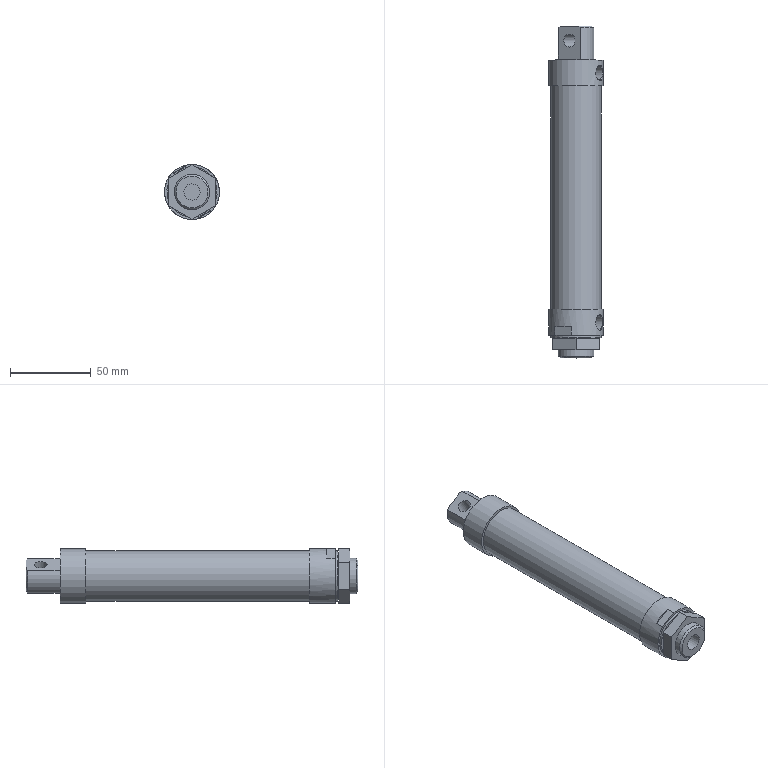Part | NX | features WGN01-25-100-Y-2-001 2 | 1 solid | 41 faces | box 34 x 205 x 34 mm | volume 131750 mm3 | plane 22 | cylinder 12 | cone 7 | commonest cylinder face diameters 22 x4 8.566 x2 31 x2 34 x2 8 x1 10 x1
STEP:
#1=CARTESIAN_POINT('',(-5.5,333.716,144.407));
#2=VERTEX_POINT('',#1);
#3=CARTESIAN_POINT('',(-0.000000942,333.716,134.881));
#4=DIRECTION('',(0.,1.,0.));
#5=DIRECTION('',(-0.5,0.,0.866));
#6=AXIS2_PLACEMENT_3D('',#3,#4,#5);
#7=CIRCLE('',#6,11.);
#8=EDGE_CURVE('',#2,#2,#7,.T.);
#9=ORIENTED_EDGE('',*,*,#8,.F.);
#10=EDGE_LOOP('',(#9));
#11=FACE_BOUND('',#10,.T.);
#12=CARTESIAN_POINT('',(-5.5,329.847,144.407));
#13=VERTEX_POINT('',#12);
#14=CARTESIAN_POINT('',(-0.000000942,329.847,134.881));
#15=DIRECTION('',(0.,1.,0.));
#16=DIRECTION('',(-0.5,0.,0.866));
#17=AXIS2_PLACEMENT_3D('',#14,#15,#16);
#18=CIRCLE('',#17,11.);
#19=EDGE_CURVE('',#13,#13,#18,.T.);
#20=ORIENTED_EDGE('',*,*,#19,.T.);
#21=EDGE_LOOP('',(#20));
#22=FACE_BOUND('',#21,.T.);
#23=CARTESIAN_POINT('',(-0.000000942,342.716,134.881));
#24=DIRECTION('',(0.,1.,0.));
#25=DIRECTION('',(0.5,0.,-0.866));
#26=AXIS2_PLACEMENT_3D('',#23,#24,#25);
#27=CYLINDRICAL_SURFACE('',#26,11.);
#28=ADVANCED_FACE('',(#11,#22),#27,.T.);
#29=ORIENTED_EDGE('',*,*,#19,.F.);
#30=EDGE_LOOP('',(#29));
#31=FACE_BOUND('',#30,.T.);
#32=CARTESIAN_POINT('',(-4.934,328.716,143.428));
#33=VERTEX_POINT('',#32);
#34=CARTESIAN_POINT('',(-0.000000942,328.716,134.881));
#35=DIRECTION('',(0.,1.,0.));
#36=DIRECTION('',(-0.5,0.,0.866));
#37=AXIS2_PLACEMENT_3D('',#34,#35,#36);
#38=CIRCLE('',#37,9.869);
#39=EDGE_CURVE('',#33,#33,#38,.T.);
#40=ORIENTED_EDGE('',*,*,#39,.T.);
#41=EDGE_LOOP('',(#40));
#42=FACE_BOUND('',#41,.T.);
#43=CARTESIAN_POINT('',(-0.000000942,328.716,134.881));
#44=DIRECTION('',(0.,1.,0.));
#45=DIRECTION('',(0.5,0.,-0.866));
#46=AXIS2_PLACEMENT_3D('',#43,#44,#45);
#47=CONICAL_SURFACE('',#46,9.869,0.7854);
#48=ADVANCED_FACE('',(#31,#42),#47,.T.);
#49=CARTESIAN_POINT('',(-2.5,512.716,139.211));
#50=VERTEX_POINT('',#49);
#51=CARTESIAN_POINT('',(-0.000000942,512.716,134.881));
#52=DIRECTION('',(0.,1.,0.));
#53=DIRECTION('',(-0.5,0.,0.866));
#54=AXIS2_PLACEMENT_3D('',#51,#52,#53);
#55=CIRCLE('',#54,5.);
#56=EDGE_CURVE('',#50,#50,#55,.T.);
#57=ORIENTED_EDGE('',*,*,#56,.T.);
#58=EDGE_LOOP('',(#57));
#59=FACE_BOUND('',#58,.T.);
#60=CARTESIAN_POINT('',(-2.5,328.716,139.211));
#61=VERTEX_POINT('',#60);
#62=CARTESIAN_POINT('',(-0.000000942,328.716,134.881));
#63=DIRECTION('',(0.,1.,0.));
#64=DIRECTION('',(-0.5,0.,0.866));
#65=AXIS2_PLACEMENT_3D('',#62,#63,#64);
#66=CIRCLE('',#65,5.);
#67=EDGE_CURVE('',#61,#61,#66,.T.);
#68=ORIENTED_EDGE('',*,*,#67,.F.);
#69=EDGE_LOOP('',(#68));
#70=FACE_BOUND('',#69,.T.);
#71=CARTESIAN_POINT('',(-0.000000942,512.716,134.881));
#72=DIRECTION('',(0.,1.,0.));
#73=DIRECTION('',(0.5,0.,-0.866));
#74=AXIS2_PLACEMENT_3D('',#71,#72,#73);
#75=CYLINDRICAL_SURFACE('',#74,5.);
#76=ADVANCED_FACE('',(#59,#70),#75,.F.);
#77=CARTESIAN_POINT('',(-7.75,342.716,148.305));
#78=VERTEX_POINT('',#77);
#79=CARTESIAN_POINT('',(-0.000000942,342.716,134.881));
#80=DIRECTION('',(0.,1.,0.));
#81=DIRECTION('',(-0.5,0.,0.866));
#82=AXIS2_PLACEMENT_3D('',#79,#80,#81);
#83=CIRCLE('',#82,15.5);
#84=EDGE_CURVE('',#78,#78,#83,.T.);
#85=ORIENTED_EDGE('',*,*,#84,.F.);
#86=EDGE_LOOP('',(#85));
#87=FACE_BOUND('',#86,.T.);
#88=CARTESIAN_POINT('',(-7.75,341.216,148.305));
#89=VERTEX_POINT('',#88);
#90=CARTESIAN_POINT('',(-0.000000942,341.216,134.881));
#91=DIRECTION('',(0.,1.,0.));
#92=DIRECTION('',(-0.5,0.,0.866));
#93=AXIS2_PLACEMENT_3D('',#90,#91,#92);
#94=CIRCLE('',#93,15.5);
#95=EDGE_CURVE('',#89,#89,#94,.T.);
#96=ORIENTED_EDGE('',*,*,#95,.T.);
#97=EDGE_LOOP('',(#96));
#98=FACE_BOUND('',#97,.T.);
#99=CARTESIAN_POINT('',(-0.000000942,342.716,134.881));
#100=DIRECTION('',(0.,1.,0.));
#101=DIRECTION('',(0.5,0.,-0.866));
#102=AXIS2_PLACEMENT_3D('',#99,#100,#101);
#103=CYLINDRICAL_SURFACE('',#102,15.5);
#104=ADVANCED_FACE('',(#87,#98),#103,.T.);
#105=CARTESIAN_POINT('',(-5.5,341.216,144.407));
#106=VERTEX_POINT('',#105);
#107=CARTESIAN_POINT('',(-0.000000942,341.216,134.881));
#108=DIRECTION('',(0.,1.,0.));
#109=DIRECTION('',(-0.5,0.,0.866));
#110=AXIS2_PLACEMENT_3D('',#107,#108,#109);
#111=CIRCLE('',#110,11.);
#112=EDGE_CURVE('',#106,#106,#111,.T.);
#113=ORIENTED_EDGE('',*,*,#112,.F.);
#114=EDGE_LOOP('',(#113));
#115=FACE_BOUND('',#114,.T.);
#116=CARTESIAN_POINT('',(-5.5,340.716,144.407));
#117=VERTEX_POINT('',#116);
#118=CARTESIAN_POINT('',(-0.000000942,340.716,134.881));
#119=DIRECTION('',(0.,1.,0.));
#120=DIRECTION('',(-0.5,0.,0.866));
#121=AXIS2_PLACEMENT_3D('',#118,#119,#120);
#122=CIRCLE('',#121,11.);
#123=EDGE_CURVE('',#117,#117,#122,.T.);
#124=ORIENTED_EDGE('',*,*,#123,.T.);
#125=EDGE_LOOP('',(#124));
#126=FACE_BOUND('',#125,.T.);
#127=CARTESIAN_POINT('',(-0.000000942,342.716,134.881));
#128=DIRECTION('',(0.,1.,0.));
#129=DIRECTION('',(0.5,0.,-0.866));
#130=AXIS2_PLACEMENT_3D('',#127,#128,#129);
#131=CYLINDRICAL_SURFACE('',#130,11.);
#132=ADVANCED_FACE('',(#115,#126),#131,.T.);
#133=CARTESIAN_POINT('',(-4.,520.716,141.809));
#134=VERTEX_POINT('',#133);
#135=CARTESIAN_POINT('',(-4.,524.716,141.809));
#136=DIRECTION('',(-0.5,0.,0.866));
#137=DIRECTION('',(0.,-1.,0.));
#138=AXIS2_PLACEMENT_3D('',#135,#136,#137);
#139=CIRCLE('',#138,4.);
#140=EDGE_CURVE('',#134,#134,#139,.T.);
#141=ORIENTED_EDGE('',*,*,#140,.T.);
#142=EDGE_LOOP('',(#141));
#143=FACE_BOUND('',#142,.T.);
#144=CARTESIAN_POINT('',(4.,520.716,127.953));
#145=VERTEX_POINT('',#144);
#146=CARTESIAN_POINT('',(4.,524.716,127.953));
#147=DIRECTION('',(-0.5,0.,0.866));
#148=DIRECTION('',(0.,-1.,0.));
#149=AXIS2_PLACEMENT_3D('',#146,#147,#148);
#150=CIRCLE('',#149,4.);
#151=EDGE_CURVE('',#145,#145,#150,.F.);
#152=ORIENTED_EDGE('',*,*,#151,.T.);
#153=EDGE_LOOP('',(#152));
#154=FACE_BOUND('',#153,.T.);
#155=CARTESIAN_POINT('',(11.,524.716,115.829));
#156=DIRECTION('',(-0.5,0.,0.866));
#157=DIRECTION('',(0.,1.,0.));
#158=AXIS2_PLACEMENT_3D('',#155,#156,#157);
#159=CYLINDRICAL_SURFACE('',#158,4.);
#160=ADVANCED_FACE('',(#143,#154),#159,.F.);
#161=CARTESIAN_POINT('',(16.396,504.716,139.372));
#162=VERTEX_POINT('',#161);
#163=CARTESIAN_POINT('',(16.248,507.739,139.997));
#164=CARTESIAN_POINT('',(16.495,504.71,138.957));
#165=CARTESIAN_POINT('',(16.248,501.709,139.993));
#166=CARTESIAN_POINT('',(15.571,500.158,141.771));
#167=CARTESIAN_POINT('',(14.763,499.703,143.38));
#168=CARTESIAN_POINT('',(13.772,500.14,144.894));
#169=CARTESIAN_POINT('',(12.557,501.689,146.391));
#170=CARTESIAN_POINT('',(11.777,504.707,147.128));
#171=CARTESIAN_POINT('',(12.548,507.718,146.4));
#172=CARTESIAN_POINT('',(13.751,509.272,144.923));
#173=CARTESIAN_POINT('',(14.741,509.729,143.417));
#174=CARTESIAN_POINT('',(15.559,509.291,141.8));
#175=CARTESIAN_POINT('',(16.248,507.739,139.997));
#176=CARTESIAN_POINT('',(16.495,504.71,138.957));
#177=CARTESIAN_POINT('',(16.248,501.709,139.993));
#178=B_SPLINE_CURVE_WITH_KNOTS('',3,(#163,#164,#165,#166,#167,#168,#169,#170,#171,#172,#173,#174,#175,#176,#177),.UNSPECIFIED.,.T.,.F.,(1,1,1,1,1,1,1,1,1,1,1,1,1,1,1,1,1,1,1),(-0.007178,-0.005384,-0.003589,0.,0.003589,0.005384,0.007178,0.008973,0.01077,0.01436,0.01795,0.01974,0.02154,0.02333,0.02512,0.02871,0.0323,0.0341,0.03589),.UNSPECIFIED.);
#179=EDGE_CURVE('',#162,#162,#178,.T.);
#180=ORIENTED_EDGE('',*,*,#179,.F.);
#181=EDGE_LOOP('',(#180));
#182=FACE_BOUND('',#181,.T.);
#183=CARTESIAN_POINT('',(16.361,504.716,139.382));
#184=VERTEX_POINT('',#183);
#185=CARTESIAN_POINT('',(14.219,504.716,143.091));
#186=DIRECTION('',(0.866,0.,0.5));
#187=DIRECTION('',(0.5,0.,-0.866));
#188=AXIS2_PLACEMENT_3D('',#185,#186,#187);
#189=CIRCLE('',#188,4.283);
#190=EDGE_CURVE('',#184,#184,#189,.T.);
#191=ORIENTED_EDGE('',*,*,#190,.F.);
#192=EDGE_LOOP('',(#191));
#193=FACE_BOUND('',#192,.T.);
#194=CARTESIAN_POINT('',(14.219,504.716,143.091));
#195=DIRECTION('',(0.866,0.,0.5));
#196=DIRECTION('',(-0.5,0.,0.866));
#197=AXIS2_PLACEMENT_3D('',#194,#195,#196);
#198=CONICAL_SURFACE('',#197,4.283,0.7854);
#199=ADVANCED_FACE('',(#182,#193),#198,.F.);
#200=ORIENTED_EDGE('',*,*,#190,.T.);
#201=EDGE_LOOP('',(#200));
#202=FACE_BOUND('',#201,.T.);
#203=CARTESIAN_POINT('',(9.503,504.716,135.422));
#204=VERTEX_POINT('',#203);
#205=CARTESIAN_POINT('',(7.361,504.716,139.131));
#206=DIRECTION('',(0.866,0.,0.5));
#207=DIRECTION('',(0.5,0.,-0.866));
#208=AXIS2_PLACEMENT_3D('',#205,#206,#207);
#209=CIRCLE('',#208,4.283);
#210=EDGE_CURVE('',#204,#204,#209,.T.);
#211=ORIENTED_EDGE('',*,*,#210,.F.);
#212=EDGE_LOOP('',(#211));
#213=FACE_BOUND('',#212,.T.);
#214=CARTESIAN_POINT('',(14.722,504.716,143.381));
#215=DIRECTION('',(0.866,0.,0.5));
#216=DIRECTION('',(-0.5,0.,0.866));
#217=AXIS2_PLACEMENT_3D('',#214,#215,#216);
#218=CYLINDRICAL_SURFACE('',#217,4.283);
#219=ADVANCED_FACE('',(#202,#213),#218,.F.);
#220=ORIENTED_EDGE('',*,*,#210,.T.);
#221=EDGE_LOOP('',(#220));
#222=FACE_BOUND('',#221,.T.);
#223=CARTESIAN_POINT('',(5.22,504.716,137.895));
#224=VERTEX_POINT('',#223);
#225=VERTEX_LOOP('',#224);
#226=FACE_BOUND('',#225,.T.);
#227=CARTESIAN_POINT('',(871.245,504.716,637.895));
#228=DIRECTION('',(0.866,0.,0.5));
#229=DIRECTION('',(-0.5,0.,0.866));
#230=AXIS2_PLACEMENT_3D('',#227,#228,#229);
#231=CONICAL_SURFACE('',#230,1732.051,1.047);
#232=ADVANCED_FACE('',(#222,#226),#231,.F.);
#233=CARTESIAN_POINT('',(5.22,350.716,142.84));
#234=VERTEX_POINT('',#233);
#235=CARTESIAN_POINT('',(7.361,350.716,139.131));
#236=DIRECTION('',(-0.866,0.,-0.5));
#237=DIRECTION('',(-0.5,0.,0.866));
#238=AXIS2_PLACEMENT_3D('',#235,#236,#237);
#239=CIRCLE('',#238,4.283);
#240=EDGE_CURVE('',#234,#234,#239,.T.);
#241=ORIENTED_EDGE('',*,*,#240,.F.);
#242=EDGE_LOOP('',(#241));
#243=FACE_BOUND('',#242,.T.);
#244=CARTESIAN_POINT('',(5.22,350.716,137.895));
#245=VERTEX_POINT('',#244);
#246=VERTEX_LOOP('',#245);
#247=FACE_BOUND('',#246,.T.);
#248=CARTESIAN_POINT('',(7.361,350.716,139.131));
#249=DIRECTION('',(0.866,0.,0.5));
#250=DIRECTION('',(-0.5,0.,0.866));
#251=AXIS2_PLACEMENT_3D('',#248,#249,#250);
#252=CONICAL_SURFACE('',#251,4.283,1.047);
#253=ADVANCED_FACE('',(#243,#247),#252,.F.);
#254=ORIENTED_EDGE('',*,*,#240,.T.);
#255=EDGE_LOOP('',(#254));
#256=FACE_BOUND('',#255,.T.);
#257=CARTESIAN_POINT('',(16.361,350.716,139.382));
#258=VERTEX_POINT('',#257);
#259=CARTESIAN_POINT('',(14.219,350.716,143.091));
#260=DIRECTION('',(0.866,0.,0.5));
#261=DIRECTION('',(0.5,0.,-0.866));
#262=AXIS2_PLACEMENT_3D('',#259,#260,#261);
#263=CIRCLE('',#262,4.283);
#264=EDGE_CURVE('',#258,#258,#263,.F.);
#265=ORIENTED_EDGE('',*,*,#264,.F.);
#266=EDGE_LOOP('',(#265));
#267=FACE_BOUND('',#266,.T.);
#268=CARTESIAN_POINT('',(7.361,350.716,139.131));
#269=DIRECTION('',(-0.866,0.,-0.5));
#270=DIRECTION('',(0.5,0.,-0.866));
#271=AXIS2_PLACEMENT_3D('',#268,#269,#270);
#272=CYLINDRICAL_SURFACE('',#271,4.283);
#273=ADVANCED_FACE('',(#256,#267),#272,.F.);
#274=CARTESIAN_POINT('',(16.396,350.716,139.372));
#275=VERTEX_POINT('',#274);
#276=CARTESIAN_POINT('',(16.248,353.739,139.997));
#277=CARTESIAN_POINT('',(16.495,350.71,138.957));
#278=CARTESIAN_POINT('',(16.248,347.709,139.993));
#279=CARTESIAN_POINT('',(15.571,346.158,141.771));
#280=CARTESIAN_POINT('',(14.763,345.703,143.38));
#281=CARTESIAN_POINT('',(13.772,346.14,144.894));
#282=CARTESIAN_POINT('',(12.557,347.689,146.391));
#283=CARTESIAN_POINT('',(11.777,350.707,147.128));
#284=CARTESIAN_POINT('',(12.548,353.718,146.4));
#285=CARTESIAN_POINT('',(13.751,355.272,144.923));
#286=CARTESIAN_POINT('',(14.741,355.729,143.417));
#287=CARTESIAN_POINT('',(15.559,355.291,141.8));
#288=CARTESIAN_POINT('',(16.248,353.739,139.997));
#289=CARTESIAN_POINT('',(16.495,350.71,138.957));
#290=CARTESIAN_POINT('',(16.248,347.709,139.993));
#291=B_SPLINE_CURVE_WITH_KNOTS('',3,(#276,#277,#278,#279,#280,#281,#282,#283,#284,#285,#286,#287,#288,#289,#290),.UNSPECIFIED.,.T.,.F.,(1,1,1,1,1,1,1,1,1,1,1,1,1,1,1,1,1,1,1),(-0.007178,-0.005384,-0.003589,0.,0.003589,0.005384,0.007178,0.008973,0.01077,0.01436,0.01795,0.01974,0.02154,0.02333,0.02512,0.02871,0.0323,0.0341,0.03589),.UNSPECIFIED.);
#292=EDGE_CURVE('',#275,#275,#291,.T.);
#293=ORIENTED_EDGE('',*,*,#292,.F.);
#294=EDGE_LOOP('',(#293));
#295=FACE_BOUND('',#294,.T.);
#296=ORIENTED_EDGE('',*,*,#264,.T.);
#297=EDGE_LOOP('',(#296));
#298=FACE_BOUND('',#297,.T.);
#299=CARTESIAN_POINT('',(14.722,350.716,143.381));
#300=DIRECTION('',(0.866,0.,0.5));
#301=DIRECTION('',(-0.5,0.,0.866));
#302=AXIS2_PLACEMENT_3D('',#299,#300,#301);
#303=CONICAL_SURFACE('',#302,4.864,0.7854);
#304=ADVANCED_FACE('',(#295,#298),#303,.F.);
#305=CARTESIAN_POINT('',(-7.75,496.716,148.305));
#306=VERTEX_POINT('',#305);
#307=CARTESIAN_POINT('',(-0.000000942,496.716,134.881));
#308=DIRECTION('',(0.,1.,0.));
#309=DIRECTION('',(-0.5,0.,0.866));
#310=AXIS2_PLACEMENT_3D('',#307,#308,#309);
#311=CIRCLE('',#310,15.5);
#312=EDGE_CURVE('',#306,#306,#311,.T.);
#313=ORIENTED_EDGE('',*,*,#312,.F.);
#314=EDGE_LOOP('',(#313));
#315=FACE_BOUND('',#314,.T.);
#316=CARTESIAN_POINT('',(-7.75,358.716,148.305));
#317=VERTEX_POINT('',#316);
#318=CARTESIAN_POINT('',(-0.000000942,358.716,134.881));
#319=DIRECTION('',(0.,1.,0.));
#320=DIRECTION('',(-0.5,0.,0.866));
#321=AXIS2_PLACEMENT_3D('',#318,#319,#320);
#322=CIRCLE('',#321,15.5);
#323=EDGE_CURVE('',#317,#317,#322,.T.);
#324=ORIENTED_EDGE('',*,*,#323,.T.);
#325=EDGE_LOOP('',(#324));
#326=FACE_BOUND('',#325,.T.);
#327=CARTESIAN_POINT('',(-0.000000942,512.716,134.881));
#328=DIRECTION('',(0.,1.,0.));
#329=DIRECTION('',(0.5,0.,-0.866));
#330=AXIS2_PLACEMENT_3D('',#327,#328,#329);
#331=CYLINDRICAL_SURFACE('',#330,15.5);
#332=ADVANCED_FACE('',(#315,#326),#331,.T.);
#333=CARTESIAN_POINT('',(-8.5,358.716,149.604));
#334=VERTEX_POINT('',#333);
#335=CARTESIAN_POINT('',(-0.000000942,358.716,134.881));
#336=DIRECTION('',(0.,1.,0.));
#337=DIRECTION('',(-0.5,0.,0.866));
#338=AXIS2_PLACEMENT_3D('',#335,#336,#337);
#339=CIRCLE('',#338,17.);
#340=EDGE_CURVE('',#334,#334,#339,.T.);
#341=ORIENTED_EDGE('',*,*,#340,.F.);
#342=EDGE_LOOP('',(#341));
#343=FACE_BOUND('',#342,.T.);
#344=ORIENTED_EDGE('',*,*,#292,.T.);
#345=EDGE_LOOP('',(#344));
#346=FACE_BOUND('',#345,.T.);
#347=CARTESIAN_POINT('',(12.975,348.049,123.897));
#348=VERTEX_POINT('',#347);
#349=CARTESIAN_POINT('',(3.025,348.049,118.153));
#350=VERTEX_POINT('',#349);
#351=CARTESIAN_POINT('',(-0.000000942,348.049,134.881));
#352=DIRECTION('',(0.,1.,0.));
#353=DIRECTION('',(0.7632,0.,-0.6461));
#354=AXIS2_PLACEMENT_3D('',#351,#352,#353);
#355=CIRCLE('',#354,17.);
#356=EDGE_CURVE('',#348,#350,#355,.T.);
#357=ORIENTED_EDGE('',*,*,#356,.T.);
#358=CARTESIAN_POINT('',(3.025,342.716,118.153));
#359=VERTEX_POINT('',#358);
#360=CARTESIAN_POINT('',(3.025,348.049,118.153));
#361=DIRECTION('',(0.,-1.,0.));
#362=VECTOR('',#361,1000.);
#363=LINE('',#360,#362);
#364=EDGE_CURVE('',#359,#350,#363,.F.);
#365=ORIENTED_EDGE('',*,*,#364,.F.);
#366=CARTESIAN_POINT('',(-12.975,342.716,145.865));
#367=VERTEX_POINT('',#366);
#368=CARTESIAN_POINT('',(-0.000000942,342.716,134.881));
#369=DIRECTION('',(0.,1.,0.));
#370=DIRECTION('',(0.1779,0.,-0.984));
#371=AXIS2_PLACEMENT_3D('',#368,#369,#370);
#372=CIRCLE('',#371,17.);
#373=EDGE_CURVE('',#359,#367,#372,.T.);
#374=ORIENTED_EDGE('',*,*,#373,.T.);
#375=CARTESIAN_POINT('',(-12.975,348.049,145.865));
#376=VERTEX_POINT('',#375);
#377=CARTESIAN_POINT('',(-12.975,348.049,145.865));
#378=DIRECTION('',(0.,-1.,0.));
#379=VECTOR('',#378,1000.);
#380=LINE('',#377,#379);
#381=EDGE_CURVE('',#367,#376,#380,.F.);
#382=ORIENTED_EDGE('',*,*,#381,.T.);
#383=CARTESIAN_POINT('',(-3.025,348.049,151.61));
#384=VERTEX_POINT('',#383);
#385=CARTESIAN_POINT('',(-0.000000942,348.049,134.881));
#386=DIRECTION('',(0.,1.,0.));
#387=DIRECTION('',(-0.7632,0.,0.6461));
#388=AXIS2_PLACEMENT_3D('',#385,#386,#387);
#389=CIRCLE('',#388,17.);
#390=EDGE_CURVE('',#376,#384,#389,.T.);
#391=ORIENTED_EDGE('',*,*,#390,.T.);
#392=CARTESIAN_POINT('',(-3.025,342.716,151.61));
#393=VERTEX_POINT('',#392);
#394=CARTESIAN_POINT('',(-3.025,348.049,151.61));
#395=DIRECTION('',(0.,-1.,0.));
#396=VECTOR('',#395,1000.);
#397=LINE('',#394,#396);
#398=EDGE_CURVE('',#384,#393,#397,.T.);
#399=ORIENTED_EDGE('',*,*,#398,.T.);
#400=CARTESIAN_POINT('',(12.975,342.716,123.897));
#401=VERTEX_POINT('',#400);
#402=CARTESIAN_POINT('',(-0.000000942,342.716,134.881));
#403=DIRECTION('',(0.,1.,0.));
#404=DIRECTION('',(-0.1779,0.,0.984));
#405=AXIS2_PLACEMENT_3D('',#402,#403,#404);
#406=CIRCLE('',#405,17.);
#407=EDGE_CURVE('',#393,#401,#406,.T.);
#408=ORIENTED_EDGE('',*,*,#407,.T.);
#409=CARTESIAN_POINT('',(12.975,348.049,123.897));
#410=DIRECTION('',(0.,-1.,0.));
#411=VECTOR('',#410,1000.);
#412=LINE('',#409,#411);
#413=EDGE_CURVE('',#348,#401,#412,.T.);
#414=ORIENTED_EDGE('',*,*,#413,.F.);
#415=EDGE_LOOP('',(#357,#365,#374,#382,#391,#399,#408,#414));
#416=FACE_BOUND('',#415,.T.);
#417=CARTESIAN_POINT('',(-0.000000942,512.716,134.881));
#418=DIRECTION('',(0.,1.,0.));
#419=DIRECTION('',(0.5,0.,-0.866));
#420=AXIS2_PLACEMENT_3D('',#417,#418,#419);
#421=CYLINDRICAL_SURFACE('',#420,17.);
#422=ADVANCED_FACE('',(#343,#346,#416),#421,.T.);
#423=CARTESIAN_POINT('',(-8.5,512.716,149.604));
#424=VERTEX_POINT('',#423);
#425=CARTESIAN_POINT('',(-0.000000942,512.716,134.881));
#426=DIRECTION('',(0.,1.,0.));
#427=DIRECTION('',(-0.5,0.,0.866));
#428=AXIS2_PLACEMENT_3D('',#425,#426,#427);
#429=CIRCLE('',#428,17.);
#430=EDGE_CURVE('',#424,#424,#429,.T.);
#431=ORIENTED_EDGE('',*,*,#430,.F.);
#432=EDGE_LOOP('',(#431));
#433=FACE_BOUND('',#432,.T.);
#434=ORIENTED_EDGE('',*,*,#179,.T.);
#435=EDGE_LOOP('',(#434));
#436=FACE_BOUND('',#435,.T.);
#437=CARTESIAN_POINT('',(-8.5,496.716,149.604));
#438=VERTEX_POINT('',#437);
#439=CARTESIAN_POINT('',(-0.000000942,496.716,134.881));
#440=DIRECTION('',(0.,1.,0.));
#441=DIRECTION('',(-0.5,0.,0.866));
#442=AXIS2_PLACEMENT_3D('',#439,#440,#441);
#443=CIRCLE('',#442,17.);
#444=EDGE_CURVE('',#438,#438,#443,.T.);
#445=ORIENTED_EDGE('',*,*,#444,.T.);
#446=EDGE_LOOP('',(#445));
#447=FACE_BOUND('',#446,.T.);
#448=CARTESIAN_POINT('',(-0.000000942,512.716,134.881));
#449=DIRECTION('',(0.,1.,0.));
#450=DIRECTION('',(0.5,0.,-0.866));
#451=AXIS2_PLACEMENT_3D('',#448,#449,#450);
#452=CYLINDRICAL_SURFACE('',#451,17.);
#453=ADVANCED_FACE('',(#433,#436,#447),#452,.T.);
#454=CARTESIAN_POINT('',(-2.538,532.584,124.178));
#455=VERTEX_POINT('',#454);
#456=CARTESIAN_POINT('',(-10.538,532.584,138.034));
#457=VERTEX_POINT('',#456);
#458=CARTESIAN_POINT('',(-0.000000942,532.584,134.881));
#459=DIRECTION('',(0.,1.,0.));
#460=DIRECTION('',(-0.2308,0.,-0.973));
#461=AXIS2_PLACEMENT_3D('',#458,#459,#460);
#462=CIRCLE('',#461,11.);
#463=EDGE_CURVE('',#455,#457,#462,.T.);
#464=ORIENTED_EDGE('',*,*,#463,.T.);
#465=CARTESIAN_POINT('',(-9.004,533.716,138.92));
#466=VERTEX_POINT('',#465);
#467=CARTESIAN_POINT('',(-10.538,532.584,138.034));
#468=CARTESIAN_POINT('',(-10.41,532.686,138.109));
#469=CARTESIAN_POINT('',(-10.218,532.836,138.219));
#470=CARTESIAN_POINT('',(-9.997,533.004,138.347));
#471=CARTESIAN_POINT('',(-9.888,533.086,138.41));
#472=CARTESIAN_POINT('',(-9.841,533.121,138.437));
#473=CARTESIAN_POINT('',(-9.81,533.144,138.455));
#474=CARTESIAN_POINT('',(-9.795,533.155,138.464));
#475=CARTESIAN_POINT('',(-9.515,533.362,138.625));
#476=CARTESIAN_POINT('',(-9.257,533.545,138.774));
#477=CARTESIAN_POINT('',(-9.004,533.716,138.92));
#478=B_SPLINE_CURVE_WITH_KNOTS('',3,(#467,#468,#469,#470,#471,#472,#473,#474,#475,#476,#477),.UNSPECIFIED.,.F.,.F.,(4,1,1,1,2,2,4),(0.,0.25,0.375,0.4375,0.4687,0.5,1.),.UNSPECIFIED.);
#479=EDGE_CURVE('',#457,#466,#478,.T.);
#480=ORIENTED_EDGE('',*,*,#479,.T.);
#481=CARTESIAN_POINT('',(-1.004,533.716,125.064));
#482=VERTEX_POINT('',#481);
#483=CARTESIAN_POINT('',(-0.000000942,533.716,134.881));
#484=DIRECTION('',(0.,1.,0.));
#485=DIRECTION('',(-0.1018,0.,-0.9948));
#486=AXIS2_PLACEMENT_3D('',#483,#484,#485);
#487=CIRCLE('',#486,9.869);
#488=EDGE_CURVE('',#482,#466,#487,.T.);
#489=ORIENTED_EDGE('',*,*,#488,.F.);
#490=CARTESIAN_POINT('',(-1.004,533.716,125.064));
#491=CARTESIAN_POINT('',(-1.132,533.63,124.99));
#492=CARTESIAN_POINT('',(-1.26,533.541,124.916));
#493=CARTESIAN_POINT('',(-1.454,533.403,124.804));
#494=CARTESIAN_POINT('',(-1.551,533.334,124.748));
#495=CARTESIAN_POINT('',(-1.649,533.262,124.692));
#496=CARTESIAN_POINT('',(-1.714,533.214,124.654));
#497=CARTESIAN_POINT('',(-1.749,533.189,124.634));
#498=CARTESIAN_POINT('',(-2.03,532.981,124.472));
#499=CARTESIAN_POINT('',(-2.283,532.787,124.326));
#500=CARTESIAN_POINT('',(-2.538,532.584,124.178));
#501=B_SPLINE_CURVE_WITH_KNOTS('',3,(#490,#491,#492,#493,#494,#495,#496,#497,#498,#499,#500),.UNSPECIFIED.,.F.,.F.,(4,2,1,2,2,4),(0.,0.25,0.375,0.4375,0.5,1.),.UNSPECIFIED.);
#502=EDGE_CURVE('',#482,#455,#501,.T.);
#503=ORIENTED_EDGE('',*,*,#502,.T.);
#504=EDGE_LOOP('',(#464,#480,#489,#503));
#505=FACE_BOUND('',#504,.T.);
#506=CARTESIAN_POINT('',(-0.000000942,532.584,134.881));
#507=DIRECTION('',(0.,-1.,0.));
#508=DIRECTION('',(-0.5,0.,0.866));
#509=AXIS2_PLACEMENT_3D('',#506,#507,#508);
#510=CONICAL_SURFACE('',#509,11.,0.7854);
#511=ADVANCED_FACE('',(#505),#510,.T.);
#512=CARTESIAN_POINT('',(-2.538,512.716,124.178));
#513=VERTEX_POINT('',#512);
#514=CARTESIAN_POINT('',(-10.538,512.716,138.034));
#515=VERTEX_POINT('',#514);
#516=CARTESIAN_POINT('',(-0.000000942,512.716,134.881));
#517=DIRECTION('',(0.,1.,0.));
#518=DIRECTION('',(-0.2308,0.,-0.973));
#519=AXIS2_PLACEMENT_3D('',#516,#517,#518);
#520=CIRCLE('',#519,11.);
#521=EDGE_CURVE('',#513,#515,#520,.T.);
#522=ORIENTED_EDGE('',*,*,#521,.T.);
#523=CARTESIAN_POINT('',(-10.538,512.716,138.034));
#524=DIRECTION('',(0.,1.,0.));
#525=VECTOR('',#524,1000.);
#526=LINE('',#523,#525);
#527=EDGE_CURVE('',#515,#457,#526,.T.);
#528=ORIENTED_EDGE('',*,*,#527,.T.);
#529=ORIENTED_EDGE('',*,*,#463,.F.);
#530=CARTESIAN_POINT('',(-2.538,512.716,124.178));
#531=DIRECTION('',(0.,1.,0.));
#532=VECTOR('',#531,1000.);
#533=LINE('',#530,#532);
#534=EDGE_CURVE('',#513,#455,#533,.T.);
#535=ORIENTED_EDGE('',*,*,#534,.F.);
#536=EDGE_LOOP('',(#522,#528,#529,#535));
#537=FACE_BOUND('',#536,.T.);
#538=CARTESIAN_POINT('',(-0.000000942,533.716,134.881));
#539=DIRECTION('',(0.,1.,0.));
#540=DIRECTION('',(0.5,0.,-0.866));
#541=AXIS2_PLACEMENT_3D('',#538,#539,#540);
#542=CYLINDRICAL_SURFACE('',#541,11.);
#543=ADVANCED_FACE('',(#537),#542,.T.);
#544=ORIENTED_EDGE('',*,*,#84,.T.);
#545=EDGE_LOOP('',(#544));
#546=FACE_BOUND('',#545,.T.);
#547=ORIENTED_EDGE('',*,*,#407,.F.);
#548=CARTESIAN_POINT('',(-3.025,342.716,151.61));
#549=DIRECTION('',(-0.866,0.,-0.5));
#550=VECTOR('',#549,1000.);
#551=LINE('',#548,#550);
#552=EDGE_CURVE('',#393,#367,#551,.T.);
#553=ORIENTED_EDGE('',*,*,#552,.T.);
#554=ORIENTED_EDGE('',*,*,#373,.F.);
#555=CARTESIAN_POINT('',(3.025,342.716,118.153));
#556=DIRECTION('',(0.866,0.,0.5));
#557=VECTOR('',#556,1000.);
#558=LINE('',#555,#557);
#559=EDGE_CURVE('',#359,#401,#558,.T.);
#560=ORIENTED_EDGE('',*,*,#559,.T.);
#561=EDGE_LOOP('',(#547,#553,#554,#560));
#562=FACE_BOUND('',#561,.T.);
#563=CARTESIAN_POINT('',(14.722,342.716,143.381));
#564=DIRECTION('',(0.,-1.,0.));
#565=DIRECTION('',(-0.5,0.,0.866));
#566=AXIS2_PLACEMENT_3D('',#563,#564,#565);
#567=PLANE('',#566);
#568=ADVANCED_FACE('',(#546,#562),#567,.T.);
#569=ORIENTED_EDGE('',*,*,#430,.T.);
#570=EDGE_LOOP('',(#569));
#571=FACE_BOUND('',#570,.T.);
#572=CARTESIAN_POINT('',(2.538,512.716,145.584));
#573=VERTEX_POINT('',#572);
#574=CARTESIAN_POINT('',(10.538,512.716,131.728));
#575=VERTEX_POINT('',#574);
#576=CARTESIAN_POINT('',(-0.000000942,512.716,134.881));
#577=DIRECTION('',(0.,1.,0.));
#578=DIRECTION('',(0.2308,0.,0.973));
#579=AXIS2_PLACEMENT_3D('',#576,#577,#578);
#580=CIRCLE('',#579,11.);
#581=EDGE_CURVE('',#573,#575,#580,.T.);
#582=ORIENTED_EDGE('',*,*,#581,.F.);
#583=CARTESIAN_POINT('',(2.538,512.716,145.584));
#584=DIRECTION('',(-0.866,0.,-0.5));
#585=VECTOR('',#584,1000.);
#586=LINE('',#583,#585);
#587=EDGE_CURVE('',#573,#515,#586,.T.);
#588=ORIENTED_EDGE('',*,*,#587,.T.);
#589=ORIENTED_EDGE('',*,*,#521,.F.);
#590=CARTESIAN_POINT('',(-2.538,512.716,124.178));
#591=DIRECTION('',(0.866,0.,0.5));
#592=VECTOR('',#591,1000.);
#593=LINE('',#590,#592);
#594=EDGE_CURVE('',#513,#575,#593,.T.);
#595=ORIENTED_EDGE('',*,*,#594,.T.);
#596=EDGE_LOOP('',(#582,#588,#589,#595));
#597=FACE_BOUND('',#596,.T.);
#598=CARTESIAN_POINT('',(4.33,512.716,137.381));
#599=DIRECTION('',(0.,1.,0.));
#600=DIRECTION('',(0.5,0.,-0.866));
#601=AXIS2_PLACEMENT_3D('',#598,#599,#600);
#602=PLANE('',#601);
#603=ADVANCED_FACE('',(#571,#597),#602,.T.);
#604=ORIENTED_EDGE('',*,*,#312,.T.);
#605=EDGE_LOOP('',(#604));
#606=FACE_BOUND('',#605,.T.);
#607=ORIENTED_EDGE('',*,*,#444,.F.);
#608=EDGE_LOOP('',(#607));
#609=FACE_BOUND('',#608,.T.);
#610=CARTESIAN_POINT('',(14.722,496.716,143.381));
#611=DIRECTION('',(0.,-1.,0.));
#612=DIRECTION('',(-0.5,0.,0.866));
#613=AXIS2_PLACEMENT_3D('',#610,#611,#612);
#614=PLANE('',#613);
#615=ADVANCED_FACE('',(#606,#609),#614,.T.);
#616=ORIENTED_EDGE('',*,*,#340,.T.);
#617=EDGE_LOOP('',(#616));
#618=FACE_BOUND('',#617,.T.);
#619=ORIENTED_EDGE('',*,*,#323,.F.);
#620=EDGE_LOOP('',(#619));
#621=FACE_BOUND('',#620,.T.);
#622=CARTESIAN_POINT('',(13.423,358.716,142.631));
#623=DIRECTION('',(0.,1.,0.));
#624=DIRECTION('',(0.5,0.,-0.866));
#625=AXIS2_PLACEMENT_3D('',#622,#623,#624);
#626=PLANE('',#625);
#627=ADVANCED_FACE('',(#618,#621),#626,.T.);
#628=ORIENTED_EDGE('',*,*,#559,.F.);
#629=ORIENTED_EDGE('',*,*,#364,.T.);
#630=CARTESIAN_POINT('',(3.025,348.049,118.153));
#631=DIRECTION('',(0.866,0.,0.5));
#632=VECTOR('',#631,1000.);
#633=LINE('',#630,#632);
#634=EDGE_CURVE('',#350,#348,#633,.T.);
#635=ORIENTED_EDGE('',*,*,#634,.T.);
#636=ORIENTED_EDGE('',*,*,#413,.T.);
#637=EDGE_LOOP('',(#628,#629,#635,#636));
#638=FACE_BOUND('',#637,.T.);
#639=CARTESIAN_POINT('',(3.025,348.049,118.153));
#640=DIRECTION('',(0.5,0.,-0.866));
#641=DIRECTION('',(0.,-1.,0.));
#642=AXIS2_PLACEMENT_3D('',#639,#640,#641);
#643=PLANE('',#642);
#644=ADVANCED_FACE('',(#638),#643,.T.);
#645=ORIENTED_EDGE('',*,*,#634,.F.);
#646=ORIENTED_EDGE('',*,*,#356,.F.);
#647=EDGE_LOOP('',(#645,#646));
#648=FACE_BOUND('',#647,.T.);
#649=CARTESIAN_POINT('',(-0.000000942,348.049,134.881));
#650=DIRECTION('',(0.,1.,0.));
#651=DIRECTION('',(0.5,0.,-0.866));
#652=AXIS2_PLACEMENT_3D('',#649,#650,#651);
#653=PLANE('',#652);
#654=ADVANCED_FACE('',(#648),#653,.F.);
#655=ORIENTED_EDGE('',*,*,#552,.F.);
#656=ORIENTED_EDGE('',*,*,#398,.F.);
#657=CARTESIAN_POINT('',(-3.025,348.049,151.61));
#658=DIRECTION('',(-0.866,0.,-0.5));
#659=VECTOR('',#658,1000.);
#660=LINE('',#657,#659);
#661=EDGE_CURVE('',#384,#376,#660,.T.);
#662=ORIENTED_EDGE('',*,*,#661,.T.);
#663=ORIENTED_EDGE('',*,*,#381,.F.);
#664=EDGE_LOOP('',(#655,#656,#662,#663));
#665=FACE_BOUND('',#664,.T.);
#666=CARTESIAN_POINT('',(-3.025,348.049,151.61));
#667=DIRECTION('',(-0.5,0.,0.866));
#668=DIRECTION('',(0.,1.,0.));
#669=AXIS2_PLACEMENT_3D('',#666,#667,#668);
#670=PLANE('',#669);
#671=ADVANCED_FACE('',(#665),#670,.T.);
#672=ORIENTED_EDGE('',*,*,#390,.F.);
#673=ORIENTED_EDGE('',*,*,#661,.F.);
#674=EDGE_LOOP('',(#672,#673));
#675=FACE_BOUND('',#674,.T.);
#676=CARTESIAN_POINT('',(-0.000000942,348.049,134.881));
#677=DIRECTION('',(0.,1.,0.));
#678=DIRECTION('',(0.5,0.,-0.866));
#679=AXIS2_PLACEMENT_3D('',#676,#677,#678);
#680=PLANE('',#679);
#681=ADVANCED_FACE('',(#675),#680,.F.);
#682=ORIENTED_EDGE('',*,*,#488,.T.);
#683=CARTESIAN_POINT('',(1.004,533.716,144.699));
#684=VERTEX_POINT('',#683);
#685=CARTESIAN_POINT('',(1.004,533.716,144.699));
#686=DIRECTION('',(-0.866,0.,-0.5));
#687=VECTOR('',#686,1000.);
#688=LINE('',#685,#687);
#689=EDGE_CURVE('',#684,#466,#688,.T.);
#690=ORIENTED_EDGE('',*,*,#689,.F.);
#691=CARTESIAN_POINT('',(9.004,533.716,130.842));
#692=VERTEX_POINT('',#691);
#693=CARTESIAN_POINT('',(-0.000000942,533.716,134.881));
#694=DIRECTION('',(0.,1.,0.));
#695=DIRECTION('',(0.1018,0.,0.9948));
#696=AXIS2_PLACEMENT_3D('',#693,#694,#695);
#697=CIRCLE('',#696,9.869);
#698=EDGE_CURVE('',#684,#692,#697,.T.);
#699=ORIENTED_EDGE('',*,*,#698,.T.);
#700=CARTESIAN_POINT('',(-1.004,533.716,125.064));
#701=DIRECTION('',(0.866,0.,0.5));
#702=VECTOR('',#701,1000.);
#703=LINE('',#700,#702);
#704=EDGE_CURVE('',#482,#692,#703,.T.);
#705=ORIENTED_EDGE('',*,*,#704,.F.);
#706=EDGE_LOOP('',(#682,#690,#699,#705));
#707=FACE_BOUND('',#706,.T.);
#708=CARTESIAN_POINT('',(8.546,533.716,139.816));
#709=DIRECTION('',(0.,-1.,0.));
#710=DIRECTION('',(-0.5,0.,0.866));
#711=AXIS2_PLACEMENT_3D('',#708,#709,#710);
#712=PLANE('',#711);
#713=ADVANCED_FACE('',(#707),#712,.F.);
#714=ORIENTED_EDGE('',*,*,#698,.F.);
#715=CARTESIAN_POINT('',(2.538,532.584,145.584));
#716=VERTEX_POINT('',#715);
#717=CARTESIAN_POINT('',(1.004,533.716,144.699));
#718=CARTESIAN_POINT('',(1.132,533.63,144.772));
#719=CARTESIAN_POINT('',(1.26,533.541,144.846));
#720=CARTESIAN_POINT('',(1.454,533.403,144.958));
#721=CARTESIAN_POINT('',(1.551,533.334,145.014));
#722=CARTESIAN_POINT('',(1.649,533.262,145.071));
#723=CARTESIAN_POINT('',(1.714,533.214,145.109));
#724=CARTESIAN_POINT('',(1.749,533.189,145.128));
#725=CARTESIAN_POINT('',(2.03,532.981,145.291));
#726=CARTESIAN_POINT('',(2.283,532.787,145.437));
#727=CARTESIAN_POINT('',(2.538,532.584,145.584));
#728=B_SPLINE_CURVE_WITH_KNOTS('',3,(#717,#718,#719,#720,#721,#722,#723,#724,#725,#726,#727),.UNSPECIFIED.,.F.,.F.,(4,2,1,2,2,4),(0.,0.25,0.375,0.4375,0.5,1.),.UNSPECIFIED.);
#729=EDGE_CURVE('',#684,#716,#728,.T.);
#730=ORIENTED_EDGE('',*,*,#729,.T.);
#731=CARTESIAN_POINT('',(10.538,532.584,131.728));
#732=VERTEX_POINT('',#731);
#733=CARTESIAN_POINT('',(-0.000000942,532.584,134.881));
#734=DIRECTION('',(0.,1.,0.));
#735=DIRECTION('',(0.2308,0.,0.973));
#736=AXIS2_PLACEMENT_3D('',#733,#734,#735);
#737=CIRCLE('',#736,11.);
#738=EDGE_CURVE('',#716,#732,#737,.T.);
#739=ORIENTED_EDGE('',*,*,#738,.T.);
#740=CARTESIAN_POINT('',(10.538,532.584,131.728));
#741=CARTESIAN_POINT('',(10.41,532.686,131.654));
#742=CARTESIAN_POINT('',(10.218,532.836,131.543));
#743=CARTESIAN_POINT('',(9.997,533.004,131.416));
#744=CARTESIAN_POINT('',(9.888,533.086,131.352));
#745=CARTESIAN_POINT('',(9.841,533.121,131.325));
#746=CARTESIAN_POINT('',(9.81,533.144,131.307));
#747=CARTESIAN_POINT('',(9.795,533.155,131.299));
#748=CARTESIAN_POINT('',(9.515,533.362,131.137));
#749=CARTESIAN_POINT('',(9.257,533.545,130.988));
#750=CARTESIAN_POINT('',(9.004,533.716,130.842));
#751=B_SPLINE_CURVE_WITH_KNOTS('',3,(#740,#741,#742,#743,#744,#745,#746,#747,#748,#749,#750),.UNSPECIFIED.,.F.,.F.,(4,1,1,1,2,2,4),(0.,0.25,0.375,0.4375,0.4688,0.5,1.),.UNSPECIFIED.);
#752=EDGE_CURVE('',#732,#692,#751,.T.);
#753=ORIENTED_EDGE('',*,*,#752,.T.);
#754=EDGE_LOOP('',(#714,#730,#739,#753));
#755=FACE_BOUND('',#754,.T.);
#756=CARTESIAN_POINT('',(-0.000000942,532.584,134.881));
#757=DIRECTION('',(0.,-1.,0.));
#758=DIRECTION('',(-0.5,0.,0.866));
#759=AXIS2_PLACEMENT_3D('',#756,#757,#758);
#760=CONICAL_SURFACE('',#759,11.,0.7854);
#761=ADVANCED_FACE('',(#755),#760,.T.);
#762=ORIENTED_EDGE('',*,*,#738,.F.);
#763=CARTESIAN_POINT('',(2.538,512.716,145.584));
#764=DIRECTION('',(0.,1.,0.));
#765=VECTOR('',#764,1000.);
#766=LINE('',#763,#765);
#767=EDGE_CURVE('',#573,#716,#766,.T.);
#768=ORIENTED_EDGE('',*,*,#767,.F.);
#769=ORIENTED_EDGE('',*,*,#581,.T.);
#770=CARTESIAN_POINT('',(10.538,512.716,131.728));
#771=DIRECTION('',(0.,1.,0.));
#772=VECTOR('',#771,1000.);
#773=LINE('',#770,#772);
#774=EDGE_CURVE('',#575,#732,#773,.T.);
#775=ORIENTED_EDGE('',*,*,#774,.T.);
#776=EDGE_LOOP('',(#762,#768,#769,#775));
#777=FACE_BOUND('',#776,.T.);
#778=CARTESIAN_POINT('',(-0.000000942,533.716,134.881));
#779=DIRECTION('',(0.,1.,0.));
#780=DIRECTION('',(0.5,0.,-0.866));
#781=AXIS2_PLACEMENT_3D('',#778,#779,#780);
#782=CYLINDRICAL_SURFACE('',#781,11.);
#783=ADVANCED_FACE('',(#777),#782,.T.);
#784=ORIENTED_EDGE('',*,*,#151,.F.);
#785=EDGE_LOOP('',(#784));
#786=FACE_BOUND('',#785,.T.);
#787=ORIENTED_EDGE('',*,*,#774,.F.);
#788=ORIENTED_EDGE('',*,*,#594,.F.);
#789=ORIENTED_EDGE('',*,*,#534,.T.);
#790=ORIENTED_EDGE('',*,*,#502,.F.);
#791=ORIENTED_EDGE('',*,*,#704,.T.);
#792=ORIENTED_EDGE('',*,*,#752,.F.);
#793=EDGE_LOOP('',(#787,#788,#789,#790,#791,#792));
#794=FACE_BOUND('',#793,.T.);
#795=CARTESIAN_POINT('',(-2.538,512.716,124.178));
#796=DIRECTION('',(-0.5,0.,0.866));
#797=DIRECTION('',(0.,1.,0.));
#798=AXIS2_PLACEMENT_3D('',#795,#796,#797);
#799=PLANE('',#798);
#800=ADVANCED_FACE('',(#786,#794),#799,.F.);
#801=ORIENTED_EDGE('',*,*,#140,.F.);
#802=EDGE_LOOP('',(#801));
#803=FACE_BOUND('',#802,.T.);
#804=ORIENTED_EDGE('',*,*,#527,.F.);
#805=ORIENTED_EDGE('',*,*,#587,.F.);
#806=ORIENTED_EDGE('',*,*,#767,.T.);
#807=ORIENTED_EDGE('',*,*,#729,.F.);
#808=ORIENTED_EDGE('',*,*,#689,.T.);
#809=ORIENTED_EDGE('',*,*,#479,.F.);
#810=EDGE_LOOP('',(#804,#805,#806,#807,#808,#809));
#811=FACE_BOUND('',#810,.T.);
#812=CARTESIAN_POINT('',(2.538,512.716,145.584));
#813=DIRECTION('',(0.5,0.,-0.866));
#814=DIRECTION('',(0.,-1.,0.));
#815=AXIS2_PLACEMENT_3D('',#812,#813,#814);
#816=PLANE('',#815);
#817=ADVANCED_FACE('',(#803,#811),#816,.F.);
#818=ORIENTED_EDGE('',*,*,#95,.F.);
#819=EDGE_LOOP('',(#818));
#820=FACE_BOUND('',#819,.T.);
#821=ORIENTED_EDGE('',*,*,#112,.T.);
#822=EDGE_LOOP('',(#821));
#823=FACE_BOUND('',#822,.T.);
#824=CARTESIAN_POINT('',(9.526,341.216,140.381));
#825=DIRECTION('',(0.,1.,0.));
#826=DIRECTION('',(0.5,0.,-0.866));
#827=AXIS2_PLACEMENT_3D('',#824,#825,#826);
#828=PLANE('',#827);
#829=ADVANCED_FACE('',(#820,#823),#828,.F.);
#830=CARTESIAN_POINT('',(14.5,340.716,126.51));
#831=VERTEX_POINT('',#830);
#832=CARTESIAN_POINT('',(-0.000000942,340.716,118.138));
#833=VERTEX_POINT('',#832);
#834=CARTESIAN_POINT('',(14.5,340.716,126.51));
#835=DIRECTION('',(-0.866,0.,-0.5));
#836=VECTOR('',#835,1000.);
#837=LINE('',#834,#836);
#838=EDGE_CURVE('',#831,#833,#837,.T.);
#839=ORIENTED_EDGE('',*,*,#838,.F.);
#840=CARTESIAN_POINT('',(14.5,333.716,126.51));
#841=VERTEX_POINT('',#840);
#842=CARTESIAN_POINT('',(14.5,333.716,126.51));
#843=DIRECTION('',(0.,1.,0.));
#844=VECTOR('',#843,1000.);
#845=LINE('',#842,#844);
#846=EDGE_CURVE('',#841,#831,#845,.T.);
#847=ORIENTED_EDGE('',*,*,#846,.F.);
#848=CARTESIAN_POINT('',(-0.000000942,333.716,118.138));
#849=VERTEX_POINT('',#848);
#850=CARTESIAN_POINT('',(14.5,333.716,126.51));
#851=DIRECTION('',(-0.866,0.,-0.5));
#852=VECTOR('',#851,1000.);
#853=LINE('',#850,#852);
#854=EDGE_CURVE('',#841,#849,#853,.T.);
#855=ORIENTED_EDGE('',*,*,#854,.T.);
#856=CARTESIAN_POINT('',(-0.000000942,333.716,118.138));
#857=DIRECTION('',(0.,1.,0.));
#858=VECTOR('',#857,1000.);
#859=LINE('',#856,#858);
#860=EDGE_CURVE('',#849,#833,#859,.T.);
#861=ORIENTED_EDGE('',*,*,#860,.T.);
#862=EDGE_LOOP('',(#839,#847,#855,#861));
#863=FACE_BOUND('',#862,.T.);
#864=CARTESIAN_POINT('',(14.5,333.716,126.51));
#865=DIRECTION('',(0.5,0.,-0.866));
#866=DIRECTION('',(0.,-1.,0.));
#867=AXIS2_PLACEMENT_3D('',#864,#865,#866);
#868=PLANE('',#867);
#869=ADVANCED_FACE('',(#863),#868,.T.);
#870=CARTESIAN_POINT('',(-14.5,340.716,126.51));
#871=VERTEX_POINT('',#870);
#872=CARTESIAN_POINT('',(-0.000000942,340.716,118.138));
#873=DIRECTION('',(-0.866,0.,0.5));
#874=VECTOR('',#873,1000.);
#875=LINE('',#872,#874);
#876=EDGE_CURVE('',#833,#871,#875,.T.);
#877=ORIENTED_EDGE('',*,*,#876,.F.);
#878=ORIENTED_EDGE('',*,*,#860,.F.);
#879=CARTESIAN_POINT('',(-14.5,333.716,126.51));
#880=VERTEX_POINT('',#879);
#881=CARTESIAN_POINT('',(-0.000000942,333.716,118.138));
#882=DIRECTION('',(-0.866,0.,0.5));
#883=VECTOR('',#882,1000.);
#884=LINE('',#881,#883);
#885=EDGE_CURVE('',#849,#880,#884,.T.);
#886=ORIENTED_EDGE('',*,*,#885,.T.);
#887=CARTESIAN_POINT('',(-14.5,333.716,126.51));
#888=DIRECTION('',(0.,1.,0.));
#889=VECTOR('',#888,1000.);
#890=LINE('',#887,#889);
#891=EDGE_CURVE('',#880,#871,#890,.T.);
#892=ORIENTED_EDGE('',*,*,#891,.T.);
#893=EDGE_LOOP('',(#877,#878,#886,#892));
#894=FACE_BOUND('',#893,.T.);
#895=CARTESIAN_POINT('',(-0.000000942,333.716,118.138));
#896=DIRECTION('',(-0.5,0.,-0.866));
#897=DIRECTION('',(0.866,0.,-0.5));
#898=AXIS2_PLACEMENT_3D('',#895,#896,#897);
#899=PLANE('',#898);
#900=ADVANCED_FACE('',(#894),#899,.T.);
#901=CARTESIAN_POINT('',(-14.5,340.716,143.253));
#902=VERTEX_POINT('',#901);
#903=CARTESIAN_POINT('',(-14.5,340.716,126.51));
#904=DIRECTION('',(0.,0.,1.));
#905=VECTOR('',#904,1000.);
#906=LINE('',#903,#905);
#907=EDGE_CURVE('',#871,#902,#906,.T.);
#908=ORIENTED_EDGE('',*,*,#907,.F.);
#909=ORIENTED_EDGE('',*,*,#891,.F.);
#910=CARTESIAN_POINT('',(-14.5,333.716,143.253));
#911=VERTEX_POINT('',#910);
#912=CARTESIAN_POINT('',(-14.5,333.716,126.51));
#913=DIRECTION('',(0.,0.,1.));
#914=VECTOR('',#913,1000.);
#915=LINE('',#912,#914);
#916=EDGE_CURVE('',#880,#911,#915,.T.);
#917=ORIENTED_EDGE('',*,*,#916,.T.);
#918=CARTESIAN_POINT('',(-14.5,333.716,143.253));
#919=DIRECTION('',(0.,1.,0.));
#920=VECTOR('',#919,1000.);
#921=LINE('',#918,#920);
#922=EDGE_CURVE('',#911,#902,#921,.T.);
#923=ORIENTED_EDGE('',*,*,#922,.T.);
#924=EDGE_LOOP('',(#908,#909,#917,#923));
#925=FACE_BOUND('',#924,.T.);
#926=CARTESIAN_POINT('',(-14.5,333.716,126.51));
#927=DIRECTION('',(-1.,0.,0.));
#928=DIRECTION('',(0.,0.,-1.));
#929=AXIS2_PLACEMENT_3D('',#926,#927,#928);
#930=PLANE('',#929);
#931=ADVANCED_FACE('',(#925),#930,.T.);
#932=CARTESIAN_POINT('',(-0.000000942,340.716,151.624));
#933=VERTEX_POINT('',#932);
#934=CARTESIAN_POINT('',(-14.5,340.716,143.253));
#935=DIRECTION('',(0.866,0.,0.5));
#936=VECTOR('',#935,1000.);
#937=LINE('',#934,#936);
#938=EDGE_CURVE('',#902,#933,#937,.T.);
#939=ORIENTED_EDGE('',*,*,#938,.F.);
#940=ORIENTED_EDGE('',*,*,#922,.F.);
#941=CARTESIAN_POINT('',(-0.000000942,333.716,151.624));
#942=VERTEX_POINT('',#941);
#943=CARTESIAN_POINT('',(-14.5,333.716,143.253));
#944=DIRECTION('',(0.866,0.,0.5));
#945=VECTOR('',#944,1000.);
#946=LINE('',#943,#945);
#947=EDGE_CURVE('',#911,#942,#946,.T.);
#948=ORIENTED_EDGE('',*,*,#947,.T.);
#949=CARTESIAN_POINT('',(-0.000000942,333.716,151.624));
#950=DIRECTION('',(0.,1.,0.));
#951=VECTOR('',#950,1000.);
#952=LINE('',#949,#951);
#953=EDGE_CURVE('',#942,#933,#952,.T.);
#954=ORIENTED_EDGE('',*,*,#953,.T.);
#955=EDGE_LOOP('',(#939,#940,#948,#954));
#956=FACE_BOUND('',#955,.T.);
#957=CARTESIAN_POINT('',(-14.5,333.716,143.253));
#958=DIRECTION('',(-0.5,0.,0.866));
#959=DIRECTION('',(0.,1.,0.));
#960=AXIS2_PLACEMENT_3D('',#957,#958,#959);
#961=PLANE('',#960);
#962=ADVANCED_FACE('',(#956),#961,.T.);
#963=CARTESIAN_POINT('',(14.5,340.716,143.253));
#964=VERTEX_POINT('',#963);
#965=CARTESIAN_POINT('',(-0.000000942,340.716,151.624));
#966=DIRECTION('',(0.866,0.,-0.5));
#967=VECTOR('',#966,1000.);
#968=LINE('',#965,#967);
#969=EDGE_CURVE('',#933,#964,#968,.T.);
#970=ORIENTED_EDGE('',*,*,#969,.F.);
#971=ORIENTED_EDGE('',*,*,#953,.F.);
#972=CARTESIAN_POINT('',(14.5,333.716,143.253));
#973=VERTEX_POINT('',#972);
#974=CARTESIAN_POINT('',(-0.000000942,333.716,151.624));
#975=DIRECTION('',(0.866,0.,-0.5));
#976=VECTOR('',#975,1000.);
#977=LINE('',#974,#976);
#978=EDGE_CURVE('',#942,#973,#977,.T.);
#979=ORIENTED_EDGE('',*,*,#978,.T.);
#980=CARTESIAN_POINT('',(14.5,333.716,143.253));
#981=DIRECTION('',(0.,1.,0.));
#982=VECTOR('',#981,1000.);
#983=LINE('',#980,#982);
#984=EDGE_CURVE('',#973,#964,#983,.T.);
#985=ORIENTED_EDGE('',*,*,#984,.T.);
#986=EDGE_LOOP('',(#970,#971,#979,#985));
#987=FACE_BOUND('',#986,.T.);
#988=CARTESIAN_POINT('',(-0.000000942,333.716,151.624));
#989=DIRECTION('',(0.5,0.,0.866));
#990=DIRECTION('',(-0.866,0.,0.5));
#991=AXIS2_PLACEMENT_3D('',#988,#989,#990);
#992=PLANE('',#991);
#993=ADVANCED_FACE('',(#987),#992,.T.);
#994=CARTESIAN_POINT('',(14.5,340.716,143.253));
#995=DIRECTION('',(0.,0.,-1.));
#996=VECTOR('',#995,1000.);
#997=LINE('',#994,#996);
#998=EDGE_CURVE('',#964,#831,#997,.T.);
#999=ORIENTED_EDGE('',*,*,#998,.F.);
#1000=ORIENTED_EDGE('',*,*,#984,.F.);
#1001=CARTESIAN_POINT('',(14.5,333.716,143.253));
#1002=DIRECTION('',(0.,0.,-1.));
#1003=VECTOR('',#1002,1000.);
#1004=LINE('',#1001,#1003);
#1005=EDGE_CURVE('',#973,#841,#1004,.T.);
#1006=ORIENTED_EDGE('',*,*,#1005,.T.);
#1007=ORIENTED_EDGE('',*,*,#846,.T.);
#1008=EDGE_LOOP('',(#999,#1000,#1006,#1007));
#1009=FACE_BOUND('',#1008,.T.);
#1010=CARTESIAN_POINT('',(14.5,333.716,143.253));
#1011=DIRECTION('',(1.,0.,0.));
#1012=DIRECTION('',(0.,0.,1.));
#1013=AXIS2_PLACEMENT_3D('',#1010,#1011,#1012);
#1014=PLANE('',#1013);
#1015=ADVANCED_FACE('',(#1009),#1014,.T.);
#1016=ORIENTED_EDGE('',*,*,#8,.T.);
#1017=EDGE_LOOP('',(#1016));
#1018=FACE_BOUND('',#1017,.T.);
#1019=ORIENTED_EDGE('',*,*,#854,.F.);
#1020=ORIENTED_EDGE('',*,*,#1005,.F.);
#1021=ORIENTED_EDGE('',*,*,#978,.F.);
#1022=ORIENTED_EDGE('',*,*,#947,.F.);
#1023=ORIENTED_EDGE('',*,*,#916,.F.);
#1024=ORIENTED_EDGE('',*,*,#885,.F.);
#1025=EDGE_LOOP('',(#1019,#1020,#1021,#1022,#1023,#1024));
#1026=FACE_BOUND('',#1025,.T.);
#1027=CARTESIAN_POINT('',(-0.000000942,333.716,134.881));
#1028=DIRECTION('',(0.,1.,0.));
#1029=DIRECTION('',(0.5,0.,-0.866));
#1030=AXIS2_PLACEMENT_3D('',#1027,#1028,#1029);
#1031=PLANE('',#1030);
#1032=ADVANCED_FACE('',(#1018,#1026),#1031,.F.);
#1033=ORIENTED_EDGE('',*,*,#123,.F.);
#1034=EDGE_LOOP('',(#1033));
#1035=FACE_BOUND('',#1034,.T.);
#1036=ORIENTED_EDGE('',*,*,#838,.T.);
#1037=ORIENTED_EDGE('',*,*,#876,.T.);
#1038=ORIENTED_EDGE('',*,*,#907,.T.);
#1039=ORIENTED_EDGE('',*,*,#938,.T.);
#1040=ORIENTED_EDGE('',*,*,#969,.T.);
#1041=ORIENTED_EDGE('',*,*,#998,.T.);
#1042=EDGE_LOOP('',(#1036,#1037,#1038,#1039,#1040,#1041));
#1043=FACE_BOUND('',#1042,.T.);
#1044=CARTESIAN_POINT('',(-0.000000942,340.716,134.881));
#1045=DIRECTION('',(0.,1.,0.));
#1046=DIRECTION('',(0.5,0.,-0.866));
#1047=AXIS2_PLACEMENT_3D('',#1044,#1045,#1046);
#1048=PLANE('',#1047);
#1049=ADVANCED_FACE('',(#1035,#1043),#1048,.T.);
#1050=ORIENTED_EDGE('',*,*,#56,.F.);
#1051=EDGE_LOOP('',(#1050));
#1052=FACE_BOUND('',#1051,.T.);
#1053=CARTESIAN_POINT('',(-0.000000942,512.716,134.881));
#1054=DIRECTION('',(0.,1.,0.));
#1055=DIRECTION('',(0.5,0.,-0.866));
#1056=AXIS2_PLACEMENT_3D('',#1053,#1054,#1055);
#1057=PLANE('',#1056);
#1058=ADVANCED_FACE('',(#1052),#1057,.F.);
#1059=ORIENTED_EDGE('',*,*,#39,.F.);
#1060=EDGE_LOOP('',(#1059));
#1061=FACE_BOUND('',#1060,.T.);
#1062=ORIENTED_EDGE('',*,*,#67,.T.);
#1063=EDGE_LOOP('',(#1062));
#1064=FACE_BOUND('',#1063,.T.);
#1065=CARTESIAN_POINT('',(-0.000000942,328.716,134.881));
#1066=DIRECTION('',(0.,1.,0.));
#1067=DIRECTION('',(0.5,0.,-0.866));
#1068=AXIS2_PLACEMENT_3D('',#1065,#1066,#1067);
#1069=PLANE('',#1068);
#1070=ADVANCED_FACE('',(#1061,#1064),#1069,.F.);
#1071=CLOSED_SHELL('',(#28,#48,#76,#104,#132,#160,#199,#219,#232,#253,#273,#304,#332,#422,#453,#511,#543,#568,#603,#615,#627,#644,#654,#671,#681,#713,#761,#783,#800,#817,#829,#869,#900,#931,#962,#993,#1015,#1032,#1049,#1058,#1070));
#1072=MANIFOLD_SOLID_BREP('',#1071);
#1073=(LENGTH_UNIT()NAMED_UNIT(*)SI_UNIT(.MILLI.,.METRE.));
#1074=UNCERTAINTY_MEASURE_WITH_UNIT(LENGTH_MEASURE(0.0508),#1073,'','');
#1075=(NAMED_UNIT(*)PLANE_ANGLE_UNIT()SI_UNIT($,.RADIAN.));
#1076=(NAMED_UNIT(*)SI_UNIT($,.STERADIAN.)SOLID_ANGLE_UNIT());
#1077=(GEOMETRIC_REPRESENTATION_CONTEXT(3)GLOBAL_UNCERTAINTY_ASSIGNED_CONTEXT((#1074))GLOBAL_UNIT_ASSIGNED_CONTEXT((#1073,#1075,#1076))REPRESENTATION_CONTEXT('',''));
#1078=ADVANCED_BREP_SHAPE_REPRESENTATION('',(#1072),#1077);